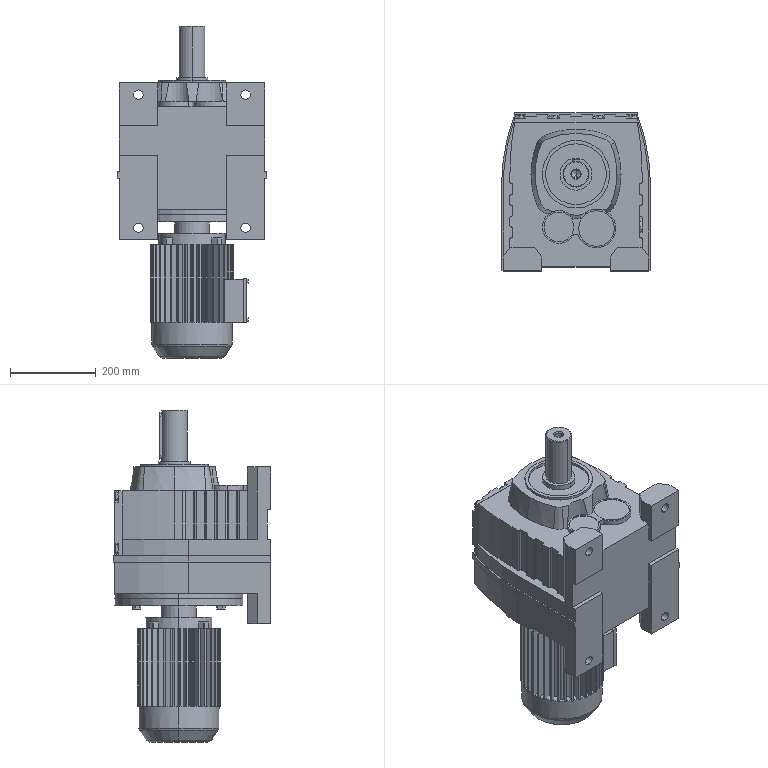Part | STEP file | R97-216.28-2.2-M1-0° R97 helical gear reducer | 2 solids | 677 faces | box 348 x 368 x 773.5 mm | volume 40162039 mm3 | plane 487 | cylinder 166 | cone 20 | torus 4 | commonest cylinder face diameters 193.4 x41 6.12 x24 3 x12 26.258 x12 7.252 x8 7.253 x8